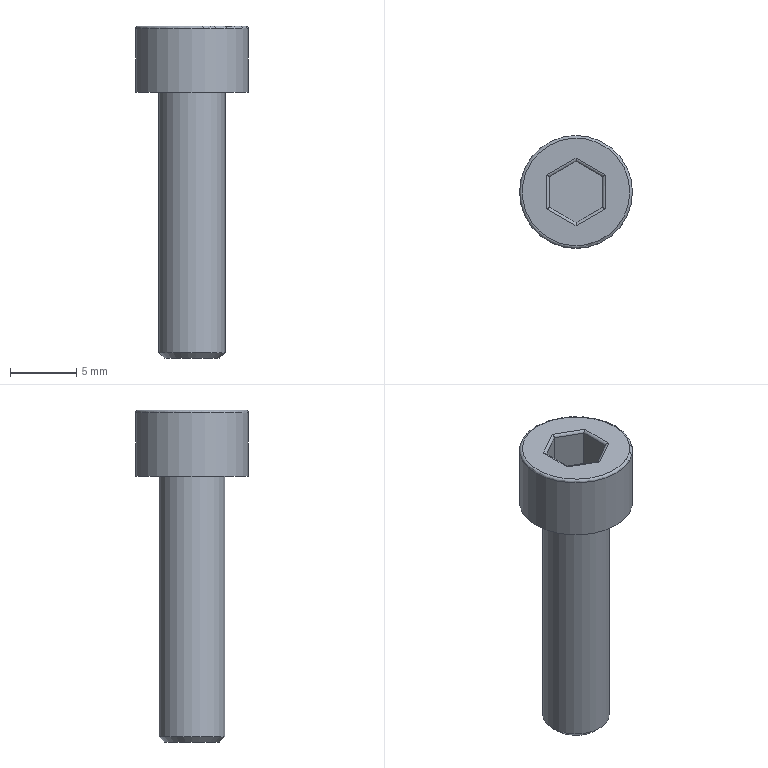Part | STEP file | 200 mesh_id738_x | 1 solid | 20 faces | box 8.5 x 8.5 x 25 mm | volume 633.317 mm3 | plane 10 | cylinder 8 | torus 1 | cone 1 | commonest cylinder face diameters 0.4 x6 5 x1 8.5 x1
STEP:
#1=CARTESIAN_POINT('',(-16876.148,-3972.269,33.1));
#2=VERTEX_POINT('',#1);
#3=CARTESIAN_POINT('',(-16873.648,-3972.269,33.1));
#4=DIRECTION('',(0.,0.,1.));
#5=DIRECTION('',(-1.,0.,0.));
#6=AXIS2_PLACEMENT_3D('',#3,#4,#5);
#7=CIRCLE('',#6,2.5);
#8=EDGE_CURVE('',#2,#2,#7,.T.);
#9=ORIENTED_EDGE('',*,*,#8,.T.);
#10=EDGE_LOOP('',(#9));
#11=FACE_BOUND('',#10,.T.);
#12=CARTESIAN_POINT('',(-16876.148,-3972.269,52.7));
#13=VERTEX_POINT('',#12);
#14=CARTESIAN_POINT('',(-16873.648,-3972.269,52.7));
#15=DIRECTION('',(0.,0.,1.));
#16=DIRECTION('',(-1.,0.,0.));
#17=AXIS2_PLACEMENT_3D('',#14,#15,#16);
#18=CIRCLE('',#17,2.5);
#19=EDGE_CURVE('',#13,#13,#18,.T.);
#20=ORIENTED_EDGE('',*,*,#19,.F.);
#21=EDGE_LOOP('',(#20));
#22=FACE_BOUND('',#21,.T.);
#23=CARTESIAN_POINT('',(-16873.648,-3972.269,52.7));
#24=DIRECTION('',(0.,0.,-1.));
#25=DIRECTION('',(1.,0.,0.));
#26=AXIS2_PLACEMENT_3D('',#23,#24,#25);
#27=CYLINDRICAL_SURFACE('',#26,2.5);
#28=ADVANCED_FACE('',(#11,#22),#27,.T.);
#29=CARTESIAN_POINT('',(-16873.648,-3969.729,57.7));
#30=VERTEX_POINT('',#29);
#31=CARTESIAN_POINT('',(-16871.448,-3970.999,57.7));
#32=VERTEX_POINT('',#31);
#33=CARTESIAN_POINT('',(-16871.548,-3970.941,57.7));
#34=DIRECTION('',(0.866,-0.5,0.));
#35=VECTOR('',#34,1.);
#36=LINE('',#33,#35);
#37=EDGE_CURVE('',#30,#32,#36,.T.);
#38=ORIENTED_EDGE('',*,*,#37,.T.);
#39=CARTESIAN_POINT('',(-16871.448,-3973.539,57.7));
#40=VERTEX_POINT('',#39);
#41=CARTESIAN_POINT('',(-16871.448,-3973.424,57.7));
#42=DIRECTION('',(0.,-1.,0.));
#43=VECTOR('',#42,1.);
#44=LINE('',#41,#43);
#45=EDGE_CURVE('',#32,#40,#44,.T.);
#46=ORIENTED_EDGE('',*,*,#45,.T.);
#47=CARTESIAN_POINT('',(-16873.648,-3974.81,57.7));
#48=VERTEX_POINT('',#47);
#49=CARTESIAN_POINT('',(-16873.548,-3974.752,57.7));
#50=DIRECTION('',(-0.866,-0.5,0.));
#51=VECTOR('',#50,1.);
#52=LINE('',#49,#51);
#53=EDGE_CURVE('',#40,#48,#52,.T.);
#54=ORIENTED_EDGE('',*,*,#53,.T.);
#55=CARTESIAN_POINT('',(-16875.848,-3973.539,57.7));
#56=VERTEX_POINT('',#55);
#57=CARTESIAN_POINT('',(-16875.748,-3973.597,57.7));
#58=DIRECTION('',(-0.866,0.5,0.));
#59=VECTOR('',#58,1.);
#60=LINE('',#57,#59);
#61=EDGE_CURVE('',#48,#56,#60,.T.);
#62=ORIENTED_EDGE('',*,*,#61,.T.);
#63=CARTESIAN_POINT('',(-16875.848,-3970.999,57.7));
#64=VERTEX_POINT('',#63);
#65=CARTESIAN_POINT('',(-16875.848,-3971.114,57.7));
#66=DIRECTION('',(0.,1.,0.));
#67=VECTOR('',#66,1.);
#68=LINE('',#65,#67);
#69=EDGE_CURVE('',#56,#64,#68,.T.);
#70=ORIENTED_EDGE('',*,*,#69,.T.);
#71=CARTESIAN_POINT('',(-16873.748,-3969.787,57.7));
#72=DIRECTION('',(0.866,0.5,0.));
#73=VECTOR('',#72,1.);
#74=LINE('',#71,#73);
#75=EDGE_CURVE('',#64,#30,#74,.T.);
#76=ORIENTED_EDGE('',*,*,#75,.T.);
#77=EDGE_LOOP('',(#38,#46,#54,#62,#70,#76));
#78=FACE_BOUND('',#77,.T.);
#79=CARTESIAN_POINT('',(-16869.598,-3972.269,57.7));
#80=VERTEX_POINT('',#79);
#81=CARTESIAN_POINT('',(-16873.648,-3972.269,57.7));
#82=DIRECTION('',(0.,0.,1.));
#83=DIRECTION('',(1.,0.,0.));
#84=AXIS2_PLACEMENT_3D('',#81,#82,#83);
#85=CIRCLE('',#84,4.05);
#86=EDGE_CURVE('',#80,#80,#85,.T.);
#87=ORIENTED_EDGE('',*,*,#86,.T.);
#88=EDGE_LOOP('',(#87));
#89=FACE_BOUND('',#88,.T.);
#90=CARTESIAN_POINT('',(-16873.648,-3972.269,57.7));
#91=DIRECTION('',(0.,0.,1.));
#92=DIRECTION('',(1.,0.,0.));
#93=AXIS2_PLACEMENT_3D('',#90,#91,#92);
#94=PLANE('',#93);
#95=ADVANCED_FACE('',(#78,#89),#94,.T.);
#96=ORIENTED_EDGE('',*,*,#19,.T.);
#97=EDGE_LOOP('',(#96));
#98=FACE_BOUND('',#97,.T.);
#99=CARTESIAN_POINT('',(-16869.398,-3972.269,52.7));
#100=VERTEX_POINT('',#99);
#101=CARTESIAN_POINT('',(-16873.648,-3972.269,52.7));
#102=DIRECTION('',(0.,0.,1.));
#103=DIRECTION('',(1.,0.,0.));
#104=AXIS2_PLACEMENT_3D('',#101,#102,#103);
#105=CIRCLE('',#104,4.25);
#106=EDGE_CURVE('',#100,#100,#105,.T.);
#107=ORIENTED_EDGE('',*,*,#106,.F.);
#108=EDGE_LOOP('',(#107));
#109=FACE_BOUND('',#108,.T.);
#110=CARTESIAN_POINT('',(-16873.648,-3972.269,52.7));
#111=DIRECTION('',(0.,0.,-1.));
#112=DIRECTION('',(-1.,0.,0.));
#113=AXIS2_PLACEMENT_3D('',#110,#111,#112);
#114=PLANE('',#113);
#115=ADVANCED_FACE('',(#98,#109),#114,.T.);
#116=CARTESIAN_POINT('',(-16869.398,-3972.269,57.5));
#117=VERTEX_POINT('',#116);
#118=CARTESIAN_POINT('',(-16873.648,-3972.269,57.5));
#119=DIRECTION('',(0.,0.,-1.));
#120=DIRECTION('',(1.,0.,0.));
#121=AXIS2_PLACEMENT_3D('',#118,#119,#120);
#122=CIRCLE('',#121,4.25);
#123=EDGE_CURVE('',#117,#117,#122,.T.);
#124=ORIENTED_EDGE('',*,*,#123,.T.);
#125=EDGE_LOOP('',(#124));
#126=FACE_BOUND('',#125,.T.);
#127=ORIENTED_EDGE('',*,*,#106,.T.);
#128=EDGE_LOOP('',(#127));
#129=FACE_BOUND('',#128,.T.);
#130=CARTESIAN_POINT('',(-16873.648,-3972.269,52.7));
#131=DIRECTION('',(0.,0.,1.));
#132=DIRECTION('',(1.,0.,0.));
#133=AXIS2_PLACEMENT_3D('',#130,#131,#132);
#134=CYLINDRICAL_SURFACE('',#133,4.25);
#135=ADVANCED_FACE('',(#126,#129),#134,.T.);
#136=ORIENTED_EDGE('',*,*,#86,.F.);
#137=EDGE_LOOP('',(#136));
#138=FACE_BOUND('',#137,.T.);
#139=ORIENTED_EDGE('',*,*,#123,.F.);
#140=EDGE_LOOP('',(#139));
#141=FACE_BOUND('',#140,.T.);
#142=CARTESIAN_POINT('',(-16873.648,-3972.269,57.5));
#143=DIRECTION('',(0.,0.,1.));
#144=DIRECTION('',(1.,0.,0.));
#145=AXIS2_PLACEMENT_3D('',#142,#143,#144);
#146=TOROIDAL_SURFACE('',#145,4.05,0.2);
#147=ADVANCED_FACE('',(#138,#141),#146,.T.);
#148=CARTESIAN_POINT('',(-16871.648,-3973.424,57.5));
#149=VERTEX_POINT('',#148);
#150=CARTESIAN_POINT('',(-16871.648,-3973.424,54.7));
#151=VERTEX_POINT('',#150);
#152=CARTESIAN_POINT('',(-16871.648,-3973.424,54.7));
#153=DIRECTION('',(0.,0.,-1.));
#154=VECTOR('',#153,1.);
#155=LINE('',#152,#154);
#156=EDGE_CURVE('',#149,#151,#155,.T.);
#157=ORIENTED_EDGE('',*,*,#156,.F.);
#158=CARTESIAN_POINT('',(-16871.648,-3971.114,57.5));
#159=VERTEX_POINT('',#158);
#160=CARTESIAN_POINT('',(-16871.648,-3971.114,57.5));
#161=DIRECTION('',(0.,1.,0.));
#162=VECTOR('',#161,1.);
#163=LINE('',#160,#162);
#164=EDGE_CURVE('',#149,#159,#163,.T.);
#165=ORIENTED_EDGE('',*,*,#164,.T.);
#166=CARTESIAN_POINT('',(-16871.648,-3971.114,54.7));
#167=VERTEX_POINT('',#166);
#168=CARTESIAN_POINT('',(-16871.648,-3971.114,54.7));
#169=DIRECTION('',(0.,0.,-1.));
#170=VECTOR('',#169,1.);
#171=LINE('',#168,#170);
#172=EDGE_CURVE('',#159,#167,#171,.T.);
#173=ORIENTED_EDGE('',*,*,#172,.T.);
#174=CARTESIAN_POINT('',(-16871.648,-3973.424,54.7));
#175=DIRECTION('',(0.,-1.,0.));
#176=VECTOR('',#175,1.);
#177=LINE('',#174,#176);
#178=EDGE_CURVE('',#167,#151,#177,.T.);
#179=ORIENTED_EDGE('',*,*,#178,.T.);
#180=EDGE_LOOP('',(#157,#165,#173,#179));
#181=FACE_OUTER_BOUND('',#180,.T.);
#182=CARTESIAN_POINT('',(-16871.648,-3973.424,54.7));
#183=DIRECTION('',(1.,0.,0.));
#184=DIRECTION('',(0.,0.,-1.));
#185=AXIS2_PLACEMENT_3D('',#182,#183,#184);
#186=PLANE('',#185);
#187=ADVANCED_FACE('',(#181),#186,.F.);
#188=ORIENTED_EDGE('',*,*,#172,.F.);
#189=CARTESIAN_POINT('',(-16873.648,-3969.96,57.5));
#190=VERTEX_POINT('',#189);
#191=CARTESIAN_POINT('',(-16873.648,-3969.96,57.5));
#192=DIRECTION('',(-0.866,0.5,0.));
#193=VECTOR('',#192,1.);
#194=LINE('',#191,#193);
#195=EDGE_CURVE('',#159,#190,#194,.T.);
#196=ORIENTED_EDGE('',*,*,#195,.T.);
#197=CARTESIAN_POINT('',(-16873.648,-3969.96,54.7));
#198=VERTEX_POINT('',#197);
#199=CARTESIAN_POINT('',(-16873.648,-3969.96,54.7));
#200=DIRECTION('',(0.,0.,-1.));
#201=VECTOR('',#200,1.);
#202=LINE('',#199,#201);
#203=EDGE_CURVE('',#190,#198,#202,.T.);
#204=ORIENTED_EDGE('',*,*,#203,.T.);
#205=CARTESIAN_POINT('',(-16871.648,-3971.114,54.7));
#206=DIRECTION('',(0.866,-0.5,0.));
#207=VECTOR('',#206,1.);
#208=LINE('',#205,#207);
#209=EDGE_CURVE('',#198,#167,#208,.T.);
#210=ORIENTED_EDGE('',*,*,#209,.T.);
#211=EDGE_LOOP('',(#188,#196,#204,#210));
#212=FACE_OUTER_BOUND('',#211,.T.);
#213=CARTESIAN_POINT('',(-16871.648,-3971.114,54.7));
#214=DIRECTION('',(0.5,0.866,0.));
#215=DIRECTION('',(-0.866,0.5,0.));
#216=AXIS2_PLACEMENT_3D('',#213,#214,#215);
#217=PLANE('',#216);
#218=ADVANCED_FACE('',(#212),#217,.F.);
#219=ORIENTED_EDGE('',*,*,#203,.F.);
#220=CARTESIAN_POINT('',(-16875.648,-3971.114,57.5));
#221=VERTEX_POINT('',#220);
#222=CARTESIAN_POINT('',(-16875.648,-3971.114,57.5));
#223=DIRECTION('',(-0.866,-0.5,0.));
#224=VECTOR('',#223,1.);
#225=LINE('',#222,#224);
#226=EDGE_CURVE('',#190,#221,#225,.T.);
#227=ORIENTED_EDGE('',*,*,#226,.T.);
#228=CARTESIAN_POINT('',(-16875.648,-3971.114,54.7));
#229=VERTEX_POINT('',#228);
#230=CARTESIAN_POINT('',(-16875.648,-3971.114,54.7));
#231=DIRECTION('',(0.,0.,-1.));
#232=VECTOR('',#231,1.);
#233=LINE('',#230,#232);
#234=EDGE_CURVE('',#221,#229,#233,.T.);
#235=ORIENTED_EDGE('',*,*,#234,.T.);
#236=CARTESIAN_POINT('',(-16873.648,-3969.96,54.7));
#237=DIRECTION('',(0.866,0.5,0.));
#238=VECTOR('',#237,1.);
#239=LINE('',#236,#238);
#240=EDGE_CURVE('',#229,#198,#239,.T.);
#241=ORIENTED_EDGE('',*,*,#240,.T.);
#242=EDGE_LOOP('',(#219,#227,#235,#241));
#243=FACE_OUTER_BOUND('',#242,.T.);
#244=CARTESIAN_POINT('',(-16873.648,-3969.96,54.7));
#245=DIRECTION('',(-0.5,0.866,0.));
#246=DIRECTION('',(-0.866,-0.5,0.));
#247=AXIS2_PLACEMENT_3D('',#244,#245,#246);
#248=PLANE('',#247);
#249=ADVANCED_FACE('',(#243),#248,.F.);
#250=ORIENTED_EDGE('',*,*,#234,.F.);
#251=CARTESIAN_POINT('',(-16875.648,-3973.424,57.5));
#252=VERTEX_POINT('',#251);
#253=CARTESIAN_POINT('',(-16875.648,-3973.424,57.5));
#254=DIRECTION('',(0.,-1.,0.));
#255=VECTOR('',#254,1.);
#256=LINE('',#253,#255);
#257=EDGE_CURVE('',#221,#252,#256,.T.);
#258=ORIENTED_EDGE('',*,*,#257,.T.);
#259=CARTESIAN_POINT('',(-16875.648,-3973.424,54.7));
#260=VERTEX_POINT('',#259);
#261=CARTESIAN_POINT('',(-16875.648,-3973.424,54.7));
#262=DIRECTION('',(0.,0.,-1.));
#263=VECTOR('',#262,1.);
#264=LINE('',#261,#263);
#265=EDGE_CURVE('',#252,#260,#264,.T.);
#266=ORIENTED_EDGE('',*,*,#265,.T.);
#267=CARTESIAN_POINT('',(-16875.648,-3971.114,54.7));
#268=DIRECTION('',(0.,1.,0.));
#269=VECTOR('',#268,1.);
#270=LINE('',#267,#269);
#271=EDGE_CURVE('',#260,#229,#270,.T.);
#272=ORIENTED_EDGE('',*,*,#271,.T.);
#273=EDGE_LOOP('',(#250,#258,#266,#272));
#274=FACE_OUTER_BOUND('',#273,.T.);
#275=CARTESIAN_POINT('',(-16875.648,-3971.114,54.7));
#276=DIRECTION('',(-1.,0.,0.));
#277=DIRECTION('',(0.,0.,1.));
#278=AXIS2_PLACEMENT_3D('',#275,#276,#277);
#279=PLANE('',#278);
#280=ADVANCED_FACE('',(#274),#279,.F.);
#281=ORIENTED_EDGE('',*,*,#265,.F.);
#282=CARTESIAN_POINT('',(-16873.648,-3974.579,57.5));
#283=VERTEX_POINT('',#282);
#284=CARTESIAN_POINT('',(-16873.648,-3974.579,57.5));
#285=DIRECTION('',(0.866,-0.5,0.));
#286=VECTOR('',#285,1.);
#287=LINE('',#284,#286);
#288=EDGE_CURVE('',#252,#283,#287,.T.);
#289=ORIENTED_EDGE('',*,*,#288,.T.);
#290=CARTESIAN_POINT('',(-16873.648,-3974.579,54.7));
#291=VERTEX_POINT('',#290);
#292=CARTESIAN_POINT('',(-16873.648,-3974.579,54.7));
#293=DIRECTION('',(0.,0.,-1.));
#294=VECTOR('',#293,1.);
#295=LINE('',#292,#294);
#296=EDGE_CURVE('',#283,#291,#295,.T.);
#297=ORIENTED_EDGE('',*,*,#296,.T.);
#298=CARTESIAN_POINT('',(-16875.648,-3973.424,54.7));
#299=DIRECTION('',(-0.866,0.5,0.));
#300=VECTOR('',#299,1.);
#301=LINE('',#298,#300);
#302=EDGE_CURVE('',#291,#260,#301,.T.);
#303=ORIENTED_EDGE('',*,*,#302,.T.);
#304=EDGE_LOOP('',(#281,#289,#297,#303));
#305=FACE_OUTER_BOUND('',#304,.T.);
#306=CARTESIAN_POINT('',(-16875.648,-3973.424,54.7));
#307=DIRECTION('',(-0.5,-0.866,0.));
#308=DIRECTION('',(0.866,-0.5,0.));
#309=AXIS2_PLACEMENT_3D('',#306,#307,#308);
#310=PLANE('',#309);
#311=ADVANCED_FACE('',(#305),#310,.F.);
#312=ORIENTED_EDGE('',*,*,#296,.F.);
#313=CARTESIAN_POINT('',(-16871.648,-3973.424,57.5));
#314=DIRECTION('',(0.866,0.5,0.));
#315=VECTOR('',#314,1.);
#316=LINE('',#313,#315);
#317=EDGE_CURVE('',#283,#149,#316,.T.);
#318=ORIENTED_EDGE('',*,*,#317,.T.);
#319=ORIENTED_EDGE('',*,*,#156,.T.);
#320=CARTESIAN_POINT('',(-16873.648,-3974.579,54.7));
#321=DIRECTION('',(-0.866,-0.5,0.));
#322=VECTOR('',#321,1.);
#323=LINE('',#320,#322);
#324=EDGE_CURVE('',#151,#291,#323,.T.);
#325=ORIENTED_EDGE('',*,*,#324,.T.);
#326=EDGE_LOOP('',(#312,#318,#319,#325));
#327=FACE_OUTER_BOUND('',#326,.T.);
#328=CARTESIAN_POINT('',(-16873.648,-3974.579,54.7));
#329=DIRECTION('',(0.5,-0.866,0.));
#330=DIRECTION('',(0.866,0.5,0.));
#331=AXIS2_PLACEMENT_3D('',#328,#329,#330);
#332=PLANE('',#331);
#333=ADVANCED_FACE('',(#327),#332,.F.);
#334=ORIENTED_EDGE('',*,*,#178,.F.);
#335=ORIENTED_EDGE('',*,*,#209,.F.);
#336=ORIENTED_EDGE('',*,*,#240,.F.);
#337=ORIENTED_EDGE('',*,*,#271,.F.);
#338=ORIENTED_EDGE('',*,*,#302,.F.);
#339=ORIENTED_EDGE('',*,*,#324,.F.);
#340=EDGE_LOOP('',(#334,#335,#336,#337,#338,#339));
#341=FACE_OUTER_BOUND('',#340,.T.);
#342=CARTESIAN_POINT('',(0.,0.,54.7));
#343=DIRECTION('',(0.,0.,1.));
#344=DIRECTION('',(1.,0.,0.));
#345=AXIS2_PLACEMENT_3D('',#342,#343,#344);
#346=PLANE('',#345);
#347=ADVANCED_FACE('',(#341),#346,.T.);
#348=CARTESIAN_POINT('',(-16875.848,-3970.999,57.5));
#349=DIRECTION('',(0.5,0.866,0.));
#350=DIRECTION('',(-0.866,0.5,0.));
#351=AXIS2_PLACEMENT_3D('',#348,#349,#350);
#352=ELLIPSE('',#351,0.2309,0.2);
#353=EDGE_CURVE('',#64,#221,#352,.T.);
#354=ORIENTED_EDGE('',*,*,#353,.F.);
#355=ORIENTED_EDGE('',*,*,#69,.F.);
#356=CARTESIAN_POINT('',(-16875.848,-3973.539,57.5));
#357=DIRECTION('',(0.5,-0.866,0.));
#358=DIRECTION('',(-0.866,-0.5,0.));
#359=AXIS2_PLACEMENT_3D('',#356,#357,#358);
#360=ELLIPSE('',#359,0.2309,0.2);
#361=EDGE_CURVE('',#252,#56,#360,.T.);
#362=ORIENTED_EDGE('',*,*,#361,.F.);
#363=ORIENTED_EDGE('',*,*,#257,.F.);
#364=EDGE_LOOP('',(#354,#355,#362,#363));
#365=FACE_OUTER_BOUND('',#364,.T.);
#366=CARTESIAN_POINT('',(-16875.848,-3971.114,57.5));
#367=DIRECTION('',(0.,1.,0.));
#368=DIRECTION('',(0.,0.,1.));
#369=AXIS2_PLACEMENT_3D('',#366,#367,#368);
#370=CYLINDRICAL_SURFACE('',#369,0.2);
#371=ADVANCED_FACE('',(#365),#370,.T.);
#372=ORIENTED_EDGE('',*,*,#361,.T.);
#373=ORIENTED_EDGE('',*,*,#61,.F.);
#374=CARTESIAN_POINT('',(-16873.648,-3974.81,57.5));
#375=DIRECTION('',(1.,0.,0.));
#376=DIRECTION('',(0.,-1.,0.));
#377=AXIS2_PLACEMENT_3D('',#374,#375,#376);
#378=ELLIPSE('',#377,0.2309,0.2);
#379=EDGE_CURVE('',#283,#48,#378,.T.);
#380=ORIENTED_EDGE('',*,*,#379,.F.);
#381=ORIENTED_EDGE('',*,*,#288,.F.);
#382=EDGE_LOOP('',(#372,#373,#380,#381));
#383=FACE_OUTER_BOUND('',#382,.T.);
#384=CARTESIAN_POINT('',(-16875.748,-3973.597,57.5));
#385=DIRECTION('',(-0.866,0.5,0.));
#386=DIRECTION('',(-0.5,-0.866,0.));
#387=AXIS2_PLACEMENT_3D('',#384,#385,#386);
#388=CYLINDRICAL_SURFACE('',#387,0.2);
#389=ADVANCED_FACE('',(#383),#388,.T.);
#390=ORIENTED_EDGE('',*,*,#353,.T.);
#391=ORIENTED_EDGE('',*,*,#226,.F.);
#392=CARTESIAN_POINT('',(-16873.648,-3969.729,57.5));
#393=DIRECTION('',(1.,0.,0.));
#394=DIRECTION('',(0.,1.,0.));
#395=AXIS2_PLACEMENT_3D('',#392,#393,#394);
#396=ELLIPSE('',#395,0.2309,0.2);
#397=EDGE_CURVE('',#30,#190,#396,.T.);
#398=ORIENTED_EDGE('',*,*,#397,.F.);
#399=ORIENTED_EDGE('',*,*,#75,.F.);
#400=EDGE_LOOP('',(#390,#391,#398,#399));
#401=FACE_OUTER_BOUND('',#400,.T.);
#402=CARTESIAN_POINT('',(-16873.748,-3969.787,57.5));
#403=DIRECTION('',(0.866,0.5,0.));
#404=DIRECTION('',(-0.5,0.866,0.));
#405=AXIS2_PLACEMENT_3D('',#402,#403,#404);
#406=CYLINDRICAL_SURFACE('',#405,0.2);
#407=ADVANCED_FACE('',(#401),#406,.T.);
#408=ORIENTED_EDGE('',*,*,#379,.T.);
#409=ORIENTED_EDGE('',*,*,#53,.F.);
#410=CARTESIAN_POINT('',(-16871.448,-3973.539,57.5));
#411=DIRECTION('',(0.5,0.866,0.));
#412=DIRECTION('',(0.866,-0.5,0.));
#413=AXIS2_PLACEMENT_3D('',#410,#411,#412);
#414=ELLIPSE('',#413,0.2309,0.2);
#415=EDGE_CURVE('',#149,#40,#414,.T.);
#416=ORIENTED_EDGE('',*,*,#415,.F.);
#417=ORIENTED_EDGE('',*,*,#317,.F.);
#418=EDGE_LOOP('',(#408,#409,#416,#417));
#419=FACE_OUTER_BOUND('',#418,.T.);
#420=CARTESIAN_POINT('',(-16873.548,-3974.752,57.5));
#421=DIRECTION('',(-0.866,-0.5,0.));
#422=DIRECTION('',(0.5,-0.866,0.));
#423=AXIS2_PLACEMENT_3D('',#420,#421,#422);
#424=CYLINDRICAL_SURFACE('',#423,0.2);
#425=ADVANCED_FACE('',(#419),#424,.T.);
#426=ORIENTED_EDGE('',*,*,#397,.T.);
#427=ORIENTED_EDGE('',*,*,#195,.F.);
#428=CARTESIAN_POINT('',(-16871.448,-3970.999,57.5));
#429=DIRECTION('',(0.5,-0.866,0.));
#430=DIRECTION('',(-0.866,-0.5,0.));
#431=AXIS2_PLACEMENT_3D('',#428,#429,#430);
#432=ELLIPSE('',#431,0.2309,0.2);
#433=EDGE_CURVE('',#32,#159,#432,.T.);
#434=ORIENTED_EDGE('',*,*,#433,.F.);
#435=ORIENTED_EDGE('',*,*,#37,.F.);
#436=EDGE_LOOP('',(#426,#427,#434,#435));
#437=FACE_OUTER_BOUND('',#436,.T.);
#438=CARTESIAN_POINT('',(-16871.548,-3970.941,57.5));
#439=DIRECTION('',(0.866,-0.5,0.));
#440=DIRECTION('',(0.5,0.866,0.));
#441=AXIS2_PLACEMENT_3D('',#438,#439,#440);
#442=CYLINDRICAL_SURFACE('',#441,0.2);
#443=ADVANCED_FACE('',(#437),#442,.T.);
#444=ORIENTED_EDGE('',*,*,#415,.T.);
#445=ORIENTED_EDGE('',*,*,#45,.F.);
#446=ORIENTED_EDGE('',*,*,#433,.T.);
#447=ORIENTED_EDGE('',*,*,#164,.F.);
#448=EDGE_LOOP('',(#444,#445,#446,#447));
#449=FACE_OUTER_BOUND('',#448,.T.);
#450=CARTESIAN_POINT('',(-16871.448,-3973.424,57.5));
#451=DIRECTION('',(0.,-1.,0.));
#452=DIRECTION('',(0.,0.,-1.));
#453=AXIS2_PLACEMENT_3D('',#450,#451,#452);
#454=CYLINDRICAL_SURFACE('',#453,0.2);
#455=ADVANCED_FACE('',(#449),#454,.T.);
#456=CARTESIAN_POINT('',(-16875.748,-3972.269,32.7));
#457=VERTEX_POINT('',#456);
#458=CARTESIAN_POINT('',(-16873.648,-3972.269,32.7));
#459=DIRECTION('',(0.,0.,-1.));
#460=DIRECTION('',(-1.,0.,0.));
#461=AXIS2_PLACEMENT_3D('',#458,#459,#460);
#462=CIRCLE('',#461,2.1);
#463=EDGE_CURVE('',#457,#457,#462,.T.);
#464=ORIENTED_EDGE('',*,*,#463,.T.);
#465=EDGE_LOOP('',(#464));
#466=FACE_OUTER_BOUND('',#465,.T.);
#467=CARTESIAN_POINT('',(-16873.648,-3972.269,32.7));
#468=DIRECTION('',(0.,0.,-1.));
#469=DIRECTION('',(-1.,0.,0.));
#470=AXIS2_PLACEMENT_3D('',#467,#468,#469);
#471=PLANE('',#470);
#472=ADVANCED_FACE('',(#466),#471,.T.);
#473=ORIENTED_EDGE('',*,*,#463,.F.);
#474=EDGE_LOOP('',(#473));
#475=FACE_BOUND('',#474,.T.);
#476=ORIENTED_EDGE('',*,*,#8,.F.);
#477=EDGE_LOOP('',(#476));
#478=FACE_BOUND('',#477,.T.);
#479=CARTESIAN_POINT('',(-16873.648,-3972.269,33.1));
#480=DIRECTION('',(0.,0.,1.));
#481=DIRECTION('',(1.,0.,0.));
#482=AXIS2_PLACEMENT_3D('',#479,#480,#481);
#483=CONICAL_SURFACE('',#482,2.5,45.);
#484=ADVANCED_FACE('',(#475,#478),#483,.T.);
#485=CLOSED_SHELL('',(#28,#95,#115,#135,#147,#187,#218,#249,#280,#311,#333,#347,#371,#389,#407,#425,#443,#455,#472,#484));
#486=MANIFOLD_SOLID_BREP('',#485);
#487=(LENGTH_UNIT()NAMED_UNIT(*)SI_UNIT(.MILLI.,.METRE.));
#488=UNCERTAINTY_MEASURE_WITH_UNIT(LENGTH_MEASURE(0.00002),#487,'','');
#489=(NAMED_UNIT(*)PLANE_ANGLE_UNIT()SI_UNIT($,.RADIAN.));
#490=PLANE_ANGLE_MEASURE_WITH_UNIT(PLANE_ANGLE_MEASURE(0.01745),#489);
#491=DIMENSIONAL_EXPONENTS(0.,0.,0.,0.,0.,0.,0.);
#492=(CONVERSION_BASED_UNIT('DEGREE',#490)NAMED_UNIT(#491)PLANE_ANGLE_UNIT());
#493=(NAMED_UNIT(*)SI_UNIT($,.STERADIAN.)SOLID_ANGLE_UNIT());
#494=(GEOMETRIC_REPRESENTATION_CONTEXT(3)GLOBAL_UNCERTAINTY_ASSIGNED_CONTEXT((#488))GLOBAL_UNIT_ASSIGNED_CONTEXT((#487,#492,#493))REPRESENTATION_CONTEXT('',''));
#495=ADVANCED_BREP_SHAPE_REPRESENTATION('',(#486),#494);